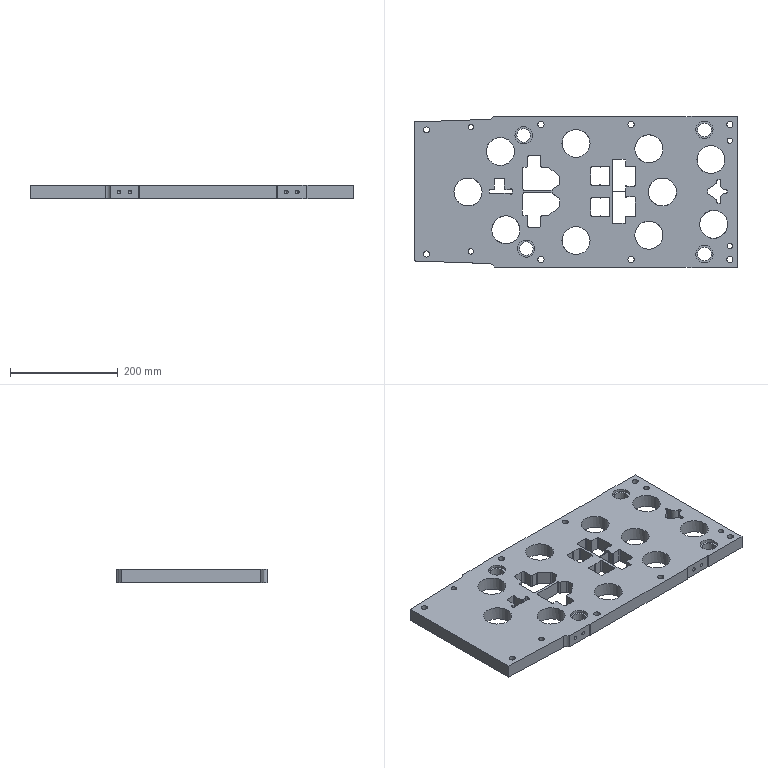Part | NX | features PH-13 2 | 1 solid | 255 faces | box 600 x 280 x 25 mm | volume 3130524 mm3 | cylinder 145 | plane 96 | cone 8 | spline 6 | commonest cylinder face diameters 4 x44 2 x14 10 x10 52.004 x10 0.6 x8 3 x8